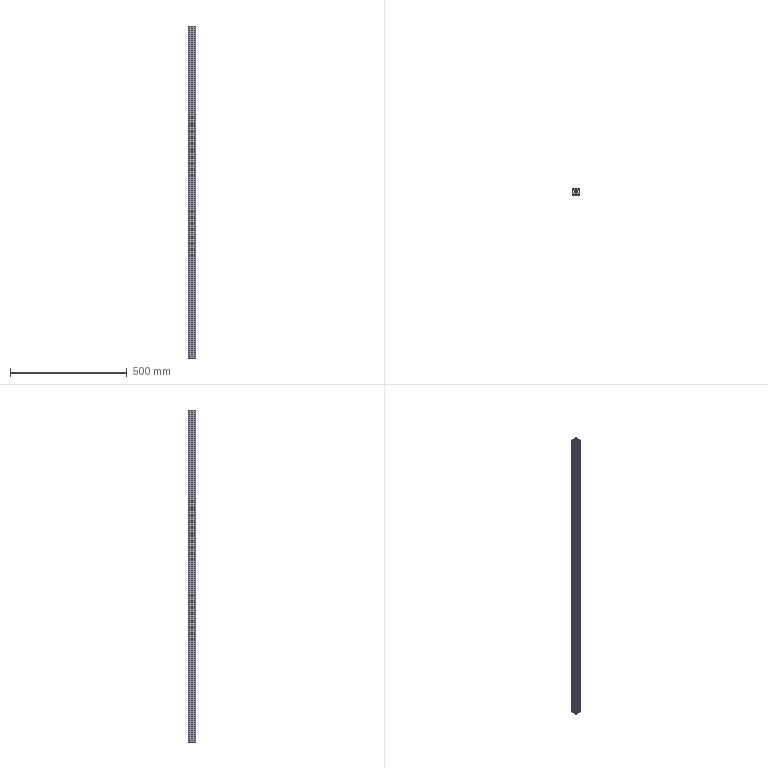Part | SolidWorks | features CirPattern 1, Extrusion 1, Fillet 1, ICE 1 | 1 solid | 60 faces | box 30 x 30 x 1420 mm | volume 556341 mm3 | plane 54 | cylinder 6 | commonest cylinder face diameters 9 x4 6.8 x2